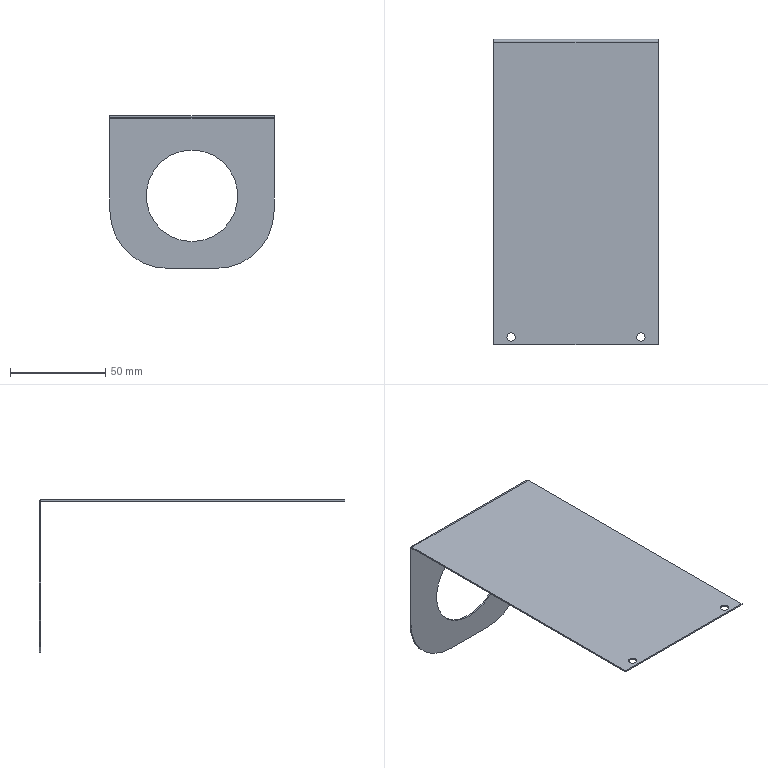Part | SolidWorks | features ICE 2, BreakCorner 1, FlatPattern 1, SMBaseFlange 1, SheetMetal 1 | 1 solid | 22 faces | box 86 x 160 x 80 mm | volume 13487 mm3 | plane 12 | cylinder 10 | commonest cylinder face diameters 4.4 x4 48 x2 60 x2 1.473 x1 2.946 x1
STEP:
#1=CARTESIAN_POINT('',(6.8,4.,-0.7366));
#2=VERTEX_POINT('',#1);
#3=CARTESIAN_POINT('',(11.2,4.,-0.7366));
#4=VERTEX_POINT('',#3);
#5=CARTESIAN_POINT('',(9.,4.,-0.7366));
#6=DIRECTION('',(0.,0.,1.));
#7=DIRECTION('',(1.,0.,0.));
#8=AXIS2_PLACEMENT_3D('',#5,#6,#7);
#9=CIRCLE('',#8,2.2);
#10=EDGE_CURVE('',#2,#4,#9,.T.);
#11=ORIENTED_EDGE('',*,*,#10,.F.);
#12=CARTESIAN_POINT('',(6.8,4.,0.));
#13=VERTEX_POINT('',#12);
#14=CARTESIAN_POINT('',(6.8,4.,-80.));
#15=DIRECTION('',(0.,0.,1.));
#16=VECTOR('',#15,1000.);
#17=LINE('',#14,#16);
#18=EDGE_CURVE('',#2,#13,#17,.T.);
#19=ORIENTED_EDGE('',*,*,#18,.T.);
#20=CARTESIAN_POINT('',(11.2,4.,0.));
#21=VERTEX_POINT('',#20);
#22=CARTESIAN_POINT('',(9.,4.,0.));
#23=DIRECTION('',(0.,0.,1.));
#24=DIRECTION('',(1.,0.,0.));
#25=AXIS2_PLACEMENT_3D('',#22,#23,#24);
#26=CIRCLE('',#25,2.2);
#27=EDGE_CURVE('',#13,#21,#26,.T.);
#28=ORIENTED_EDGE('',*,*,#27,.T.);
#29=CARTESIAN_POINT('',(11.2,4.,-80.));
#30=DIRECTION('',(0.,0.,1.));
#31=VECTOR('',#30,1000.);
#32=LINE('',#29,#31);
#33=EDGE_CURVE('',#4,#21,#32,.T.);
#34=ORIENTED_EDGE('',*,*,#33,.F.);
#35=EDGE_LOOP('',(#11,#19,#28,#34));
#36=FACE_OUTER_BOUND('',#35,.T.);
#37=CARTESIAN_POINT('',(9.,4.,-80.));
#38=DIRECTION('',(0.,0.,1.));
#39=DIRECTION('',(1.,0.,0.));
#40=AXIS2_PLACEMENT_3D('',#37,#38,#39);
#41=CYLINDRICAL_SURFACE('',#40,2.2);
#42=ADVANCED_FACE('',(#36),#41,.F.);
#43=CARTESIAN_POINT('',(74.8,4.,-0.7366));
#44=VERTEX_POINT('',#43);
#45=CARTESIAN_POINT('',(79.2,4.,-0.7366));
#46=VERTEX_POINT('',#45);
#47=CARTESIAN_POINT('',(77.,4.,-0.7366));
#48=DIRECTION('',(0.,0.,1.));
#49=DIRECTION('',(1.,0.,0.));
#50=AXIS2_PLACEMENT_3D('',#47,#48,#49);
#51=CIRCLE('',#50,2.2);
#52=EDGE_CURVE('',#44,#46,#51,.T.);
#53=ORIENTED_EDGE('',*,*,#52,.F.);
#54=CARTESIAN_POINT('',(74.8,4.,0.));
#55=VERTEX_POINT('',#54);
#56=CARTESIAN_POINT('',(74.8,4.,-80.));
#57=DIRECTION('',(0.,0.,1.));
#58=VECTOR('',#57,1000.);
#59=LINE('',#56,#58);
#60=EDGE_CURVE('',#44,#55,#59,.T.);
#61=ORIENTED_EDGE('',*,*,#60,.T.);
#62=CARTESIAN_POINT('',(79.2,4.,0.));
#63=VERTEX_POINT('',#62);
#64=CARTESIAN_POINT('',(77.,4.,0.));
#65=DIRECTION('',(0.,0.,1.));
#66=DIRECTION('',(1.,0.,0.));
#67=AXIS2_PLACEMENT_3D('',#64,#65,#66);
#68=CIRCLE('',#67,2.2);
#69=EDGE_CURVE('',#55,#63,#68,.T.);
#70=ORIENTED_EDGE('',*,*,#69,.T.);
#71=CARTESIAN_POINT('',(79.2,4.,-80.));
#72=DIRECTION('',(0.,0.,1.));
#73=VECTOR('',#72,1000.);
#74=LINE('',#71,#73);
#75=EDGE_CURVE('',#46,#63,#74,.T.);
#76=ORIENTED_EDGE('',*,*,#75,.F.);
#77=EDGE_LOOP('',(#53,#61,#70,#76));
#78=FACE_OUTER_BOUND('',#77,.T.);
#79=CARTESIAN_POINT('',(77.,4.,-80.));
#80=DIRECTION('',(0.,0.,1.));
#81=DIRECTION('',(1.,0.,0.));
#82=AXIS2_PLACEMENT_3D('',#79,#80,#81);
#83=CYLINDRICAL_SURFACE('',#82,2.2);
#84=ADVANCED_FACE('',(#78),#83,.F.);
#85=CARTESIAN_POINT('',(43.,159.263,-66.));
#86=VERTEX_POINT('',#85);
#87=CARTESIAN_POINT('',(43.,159.263,-18.));
#88=VERTEX_POINT('',#87);
#89=CARTESIAN_POINT('',(43.,159.263,-42.));
#90=DIRECTION('',(0.,1.,0.));
#91=DIRECTION('',(0.,0.,1.));
#92=AXIS2_PLACEMENT_3D('',#89,#90,#91);
#93=CIRCLE('',#92,24.);
#94=EDGE_CURVE('',#86,#88,#93,.T.);
#95=ORIENTED_EDGE('',*,*,#94,.F.);
#96=CARTESIAN_POINT('',(43.,160.,-66.));
#97=VERTEX_POINT('',#96);
#98=CARTESIAN_POINT('',(43.,150.,-66.));
#99=DIRECTION('',(0.,1.,0.));
#100=VECTOR('',#99,1000.);
#101=LINE('',#98,#100);
#102=EDGE_CURVE('',#86,#97,#101,.T.);
#103=ORIENTED_EDGE('',*,*,#102,.T.);
#104=CARTESIAN_POINT('',(43.,160.,-18.));
#105=VERTEX_POINT('',#104);
#106=CARTESIAN_POINT('',(43.,160.,-42.));
#107=DIRECTION('',(0.,1.,0.));
#108=DIRECTION('',(0.,0.,1.));
#109=AXIS2_PLACEMENT_3D('',#106,#107,#108);
#110=CIRCLE('',#109,24.);
#111=EDGE_CURVE('',#97,#105,#110,.T.);
#112=ORIENTED_EDGE('',*,*,#111,.T.);
#113=CARTESIAN_POINT('',(43.,150.,-18.));
#114=DIRECTION('',(0.,1.,0.));
#115=VECTOR('',#114,1000.);
#116=LINE('',#113,#115);
#117=EDGE_CURVE('',#88,#105,#116,.T.);
#118=ORIENTED_EDGE('',*,*,#117,.F.);
#119=EDGE_LOOP('',(#95,#103,#112,#118));
#120=FACE_OUTER_BOUND('',#119,.T.);
#121=CARTESIAN_POINT('',(43.,150.,-42.));
#122=DIRECTION('',(0.,1.,0.));
#123=DIRECTION('',(0.,0.,1.));
#124=AXIS2_PLACEMENT_3D('',#121,#122,#123);
#125=CYLINDRICAL_SURFACE('',#124,24.);
#126=ADVANCED_FACE('',(#120),#125,.F.);
#127=CARTESIAN_POINT('',(86.,160.,-1.473));
#128=VERTEX_POINT('',#127);
#129=CARTESIAN_POINT('',(86.,159.263,-1.473));
#130=VERTEX_POINT('',#129);
#131=CARTESIAN_POINT('',(86.,160.,-1.473));
#132=DIRECTION('',(0.,-1.,0.));
#133=VECTOR('',#132,1000.);
#134=LINE('',#131,#133);
#135=EDGE_CURVE('',#128,#130,#134,.T.);
#136=ORIENTED_EDGE('',*,*,#135,.F.);
#137=CARTESIAN_POINT('',(86.,158.527,0.));
#138=VERTEX_POINT('',#137);
#139=CARTESIAN_POINT('',(86.,158.527,-1.473));
#140=DIRECTION('',(-1.,0.,0.));
#141=DIRECTION('',(0.,0.,-1.));
#142=AXIS2_PLACEMENT_3D('',#139,#140,#141);
#143=CIRCLE('',#142,1.473);
#144=EDGE_CURVE('',#138,#128,#143,.T.);
#145=ORIENTED_EDGE('',*,*,#144,.F.);
#146=CARTESIAN_POINT('',(86.,158.527,-0.7366));
#147=VERTEX_POINT('',#146);
#148=CARTESIAN_POINT('',(86.,158.527,-0.7366));
#149=DIRECTION('',(0.,0.,1.));
#150=VECTOR('',#149,1000.);
#151=LINE('',#148,#150);
#152=EDGE_CURVE('',#147,#138,#151,.T.);
#153=ORIENTED_EDGE('',*,*,#152,.F.);
#154=CARTESIAN_POINT('',(86.,158.527,-1.473));
#155=DIRECTION('',(-1.,0.,0.));
#156=DIRECTION('',(0.,0.,-1.));
#157=AXIS2_PLACEMENT_3D('',#154,#155,#156);
#158=CIRCLE('',#157,0.7366);
#159=EDGE_CURVE('',#147,#130,#158,.T.);
#160=ORIENTED_EDGE('',*,*,#159,.T.);
#161=EDGE_LOOP('',(#136,#145,#153,#160));
#162=FACE_OUTER_BOUND('',#161,.T.);
#163=CARTESIAN_POINT('',(86.,160.,-1.473));
#164=DIRECTION('',(1.,0.,0.));
#165=DIRECTION('',(0.,0.,-1.));
#166=AXIS2_PLACEMENT_3D('',#163,#164,#165);
#167=PLANE('',#166);
#168=ADVANCED_FACE('',(#162),#167,.T.);
#169=CARTESIAN_POINT('',(86.,159.263,-50.));
#170=VERTEX_POINT('',#169);
#171=CARTESIAN_POINT('',(86.,159.263,0.));
#172=DIRECTION('',(0.,0.,-1.));
#173=VECTOR('',#172,1000.);
#174=LINE('',#171,#173);
#175=EDGE_CURVE('',#130,#170,#174,.T.);
#176=ORIENTED_EDGE('',*,*,#175,.T.);
#177=CARTESIAN_POINT('',(86.,160.,-50.));
#178=VERTEX_POINT('',#177);
#179=CARTESIAN_POINT('',(86.,158.527,-50.));
#180=DIRECTION('',(0.,1.,0.));
#181=VECTOR('',#180,1000.);
#182=LINE('',#179,#181);
#183=EDGE_CURVE('',#170,#178,#182,.T.);
#184=ORIENTED_EDGE('',*,*,#183,.T.);
#185=CARTESIAN_POINT('',(86.,160.,0.));
#186=DIRECTION('',(0.,0.,-1.));
#187=VECTOR('',#186,1000.);
#188=LINE('',#185,#187);
#189=EDGE_CURVE('',#128,#178,#188,.T.);
#190=ORIENTED_EDGE('',*,*,#189,.F.);
#191=ORIENTED_EDGE('',*,*,#135,.T.);
#192=EDGE_LOOP('',(#176,#184,#190,#191));
#193=FACE_OUTER_BOUND('',#192,.T.);
#194=CARTESIAN_POINT('',(86.,158.527,-0.7366));
#195=DIRECTION('',(1.,0.,0.));
#196=DIRECTION('',(0.,0.,-1.));
#197=AXIS2_PLACEMENT_3D('',#194,#195,#196);
#198=PLANE('',#197);
#199=ADVANCED_FACE('',(#193),#198,.T.);
#200=CARTESIAN_POINT('',(0.,158.527,0.));
#201=VERTEX_POINT('',#200);
#202=CARTESIAN_POINT('',(0.,158.527,-0.7366));
#203=VERTEX_POINT('',#202);
#204=CARTESIAN_POINT('',(0.,158.527,0.));
#205=DIRECTION('',(0.,0.,-1.));
#206=VECTOR('',#205,1000.);
#207=LINE('',#204,#206);
#208=EDGE_CURVE('',#201,#203,#207,.T.);
#209=ORIENTED_EDGE('',*,*,#208,.F.);
#210=CARTESIAN_POINT('',(0.,160.,-1.473));
#211=VERTEX_POINT('',#210);
#212=CARTESIAN_POINT('',(0.,158.527,-1.473));
#213=DIRECTION('',(-1.,0.,0.));
#214=DIRECTION('',(0.,0.,-1.));
#215=AXIS2_PLACEMENT_3D('',#212,#213,#214);
#216=CIRCLE('',#215,1.473);
#217=EDGE_CURVE('',#201,#211,#216,.T.);
#218=ORIENTED_EDGE('',*,*,#217,.T.);
#219=CARTESIAN_POINT('',(0.,159.263,-1.473));
#220=VERTEX_POINT('',#219);
#221=CARTESIAN_POINT('',(0.,159.263,-1.473));
#222=DIRECTION('',(0.,1.,0.));
#223=VECTOR('',#222,1000.);
#224=LINE('',#221,#223);
#225=EDGE_CURVE('',#220,#211,#224,.T.);
#226=ORIENTED_EDGE('',*,*,#225,.F.);
#227=CARTESIAN_POINT('',(0.,158.527,-1.473));
#228=DIRECTION('',(-1.,0.,0.));
#229=DIRECTION('',(0.,0.,-1.));
#230=AXIS2_PLACEMENT_3D('',#227,#228,#229);
#231=CIRCLE('',#230,0.7366);
#232=EDGE_CURVE('',#203,#220,#231,.T.);
#233=ORIENTED_EDGE('',*,*,#232,.F.);
#234=EDGE_LOOP('',(#209,#218,#226,#233));
#235=FACE_OUTER_BOUND('',#234,.T.);
#236=CARTESIAN_POINT('',(0.,158.527,0.));
#237=DIRECTION('',(-1.,0.,0.));
#238=DIRECTION('',(0.,0.,1.));
#239=AXIS2_PLACEMENT_3D('',#236,#237,#238);
#240=PLANE('',#239);
#241=ADVANCED_FACE('',(#235),#240,.T.);
#242=CARTESIAN_POINT('',(0.,0.,0.));
#243=VERTEX_POINT('',#242);
#244=CARTESIAN_POINT('',(0.,0.,0.));
#245=DIRECTION('',(0.,1.,0.));
#246=VECTOR('',#245,1000.);
#247=LINE('',#244,#246);
#248=EDGE_CURVE('',#243,#201,#247,.T.);
#249=ORIENTED_EDGE('',*,*,#248,.T.);
#250=ORIENTED_EDGE('',*,*,#208,.T.);
#251=CARTESIAN_POINT('',(0.,0.,-0.7366));
#252=VERTEX_POINT('',#251);
#253=CARTESIAN_POINT('',(0.,0.,-0.7366));
#254=DIRECTION('',(0.,1.,0.));
#255=VECTOR('',#254,1000.);
#256=LINE('',#253,#255);
#257=EDGE_CURVE('',#252,#203,#256,.T.);
#258=ORIENTED_EDGE('',*,*,#257,.F.);
#259=CARTESIAN_POINT('',(0.,0.,-0.7366));
#260=DIRECTION('',(0.,0.,1.));
#261=VECTOR('',#260,1000.);
#262=LINE('',#259,#261);
#263=EDGE_CURVE('',#252,#243,#262,.T.);
#264=ORIENTED_EDGE('',*,*,#263,.T.);
#265=EDGE_LOOP('',(#249,#250,#258,#264));
#266=FACE_OUTER_BOUND('',#265,.T.);
#267=CARTESIAN_POINT('',(0.,159.263,-1.473));
#268=DIRECTION('',(-1.,0.,0.));
#269=DIRECTION('',(0.,0.,1.));
#270=AXIS2_PLACEMENT_3D('',#267,#268,#269);
#271=PLANE('',#270);
#272=ADVANCED_FACE('',(#266),#271,.T.);
#273=CARTESIAN_POINT('',(43.,159.263,-42.));
#274=DIRECTION('',(0.,1.,0.));
#275=DIRECTION('',(0.,0.,1.));
#276=AXIS2_PLACEMENT_3D('',#273,#274,#275);
#277=CIRCLE('',#276,24.);
#278=EDGE_CURVE('',#88,#86,#277,.T.);
#279=ORIENTED_EDGE('',*,*,#278,.T.);
#280=ORIENTED_EDGE('',*,*,#94,.T.);
#281=EDGE_LOOP('',(#279,#280));
#282=FACE_BOUND('',#281,.T.);
#283=CARTESIAN_POINT('',(56.,159.263,-80.));
#284=VERTEX_POINT('',#283);
#285=CARTESIAN_POINT('',(30.,159.263,-80.));
#286=VERTEX_POINT('',#285);
#287=CARTESIAN_POINT('',(86.,159.263,-80.));
#288=DIRECTION('',(-1.,0.,0.));
#289=VECTOR('',#288,1000.);
#290=LINE('',#287,#289);
#291=EDGE_CURVE('',#284,#286,#290,.T.);
#292=ORIENTED_EDGE('',*,*,#291,.F.);
#293=CARTESIAN_POINT('',(56.,159.263,-50.));
#294=DIRECTION('',(0.,-1.,0.));
#295=DIRECTION('',(0.,0.,1.));
#296=AXIS2_PLACEMENT_3D('',#293,#294,#295);
#297=CIRCLE('',#296,30.);
#298=EDGE_CURVE('',#284,#170,#297,.T.);
#299=ORIENTED_EDGE('',*,*,#298,.T.);
#300=ORIENTED_EDGE('',*,*,#175,.F.);
#301=CARTESIAN_POINT('',(86.,159.263,-1.473));
#302=DIRECTION('',(-1.,0.,0.));
#303=VECTOR('',#302,1000.);
#304=LINE('',#301,#303);
#305=EDGE_CURVE('',#130,#220,#304,.T.);
#306=ORIENTED_EDGE('',*,*,#305,.T.);
#307=CARTESIAN_POINT('',(0.,159.263,-50.));
#308=VERTEX_POINT('',#307);
#309=CARTESIAN_POINT('',(0.,159.263,0.));
#310=DIRECTION('',(0.,0.,-1.));
#311=VECTOR('',#310,1000.);
#312=LINE('',#309,#311);
#313=EDGE_CURVE('',#220,#308,#312,.T.);
#314=ORIENTED_EDGE('',*,*,#313,.T.);
#315=CARTESIAN_POINT('',(30.,159.263,-50.));
#316=DIRECTION('',(0.,-1.,0.));
#317=DIRECTION('',(0.,0.,1.));
#318=AXIS2_PLACEMENT_3D('',#315,#316,#317);
#319=CIRCLE('',#318,30.);
#320=EDGE_CURVE('',#308,#286,#319,.T.);
#321=ORIENTED_EDGE('',*,*,#320,.T.);
#322=EDGE_LOOP('',(#292,#299,#300,#306,#314,#321));
#323=FACE_OUTER_BOUND('',#322,.T.);
#324=CARTESIAN_POINT('',(86.,159.263,0.));
#325=DIRECTION('',(0.,1.,0.));
#326=DIRECTION('',(0.,0.,1.));
#327=AXIS2_PLACEMENT_3D('',#324,#325,#326);
#328=PLANE('',#327);
#329=ADVANCED_FACE('',(#282,#323),#328,.F.);
#330=CARTESIAN_POINT('',(56.,160.,-80.));
#331=VERTEX_POINT('',#330);
#332=CARTESIAN_POINT('',(30.,160.,-80.));
#333=VERTEX_POINT('',#332);
#334=CARTESIAN_POINT('',(86.,160.,-80.));
#335=DIRECTION('',(-1.,0.,0.));
#336=VECTOR('',#335,1000.);
#337=LINE('',#334,#336);
#338=EDGE_CURVE('',#331,#333,#337,.T.);
#339=ORIENTED_EDGE('',*,*,#338,.F.);
#340=CARTESIAN_POINT('',(56.,160.,-80.));
#341=DIRECTION('',(0.,-1.,0.));
#342=VECTOR('',#341,1000.);
#343=LINE('',#340,#342);
#344=EDGE_CURVE('',#331,#284,#343,.T.);
#345=ORIENTED_EDGE('',*,*,#344,.T.);
#346=ORIENTED_EDGE('',*,*,#291,.T.);
#347=CARTESIAN_POINT('',(30.,160.,-80.));
#348=DIRECTION('',(0.,1.,0.));
#349=VECTOR('',#348,1000.);
#350=LINE('',#347,#349);
#351=EDGE_CURVE('',#286,#333,#350,.T.);
#352=ORIENTED_EDGE('',*,*,#351,.T.);
#353=EDGE_LOOP('',(#339,#345,#346,#352));
#354=FACE_OUTER_BOUND('',#353,.T.);
#355=CARTESIAN_POINT('',(86.,160.,-80.));
#356=DIRECTION('',(0.,0.,-1.));
#357=DIRECTION('',(-1.,0.,0.));
#358=AXIS2_PLACEMENT_3D('',#355,#356,#357);
#359=PLANE('',#358);
#360=ADVANCED_FACE('',(#354),#359,.T.);
#361=CARTESIAN_POINT('',(43.,160.,-42.));
#362=DIRECTION('',(0.,1.,0.));
#363=DIRECTION('',(0.,0.,1.));
#364=AXIS2_PLACEMENT_3D('',#361,#362,#363);
#365=CIRCLE('',#364,24.);
#366=EDGE_CURVE('',#105,#97,#365,.T.);
#367=ORIENTED_EDGE('',*,*,#366,.F.);
#368=ORIENTED_EDGE('',*,*,#111,.F.);
#369=EDGE_LOOP('',(#367,#368));
#370=FACE_BOUND('',#369,.T.);
#371=ORIENTED_EDGE('',*,*,#189,.T.);
#372=CARTESIAN_POINT('',(56.,160.,-50.));
#373=DIRECTION('',(0.,1.,0.));
#374=DIRECTION('',(0.,0.,1.));
#375=AXIS2_PLACEMENT_3D('',#372,#373,#374);
#376=CIRCLE('',#375,30.);
#377=EDGE_CURVE('',#178,#331,#376,.T.);
#378=ORIENTED_EDGE('',*,*,#377,.T.);
#379=ORIENTED_EDGE('',*,*,#338,.T.);
#380=CARTESIAN_POINT('',(0.,160.,-50.));
#381=VERTEX_POINT('',#380);
#382=CARTESIAN_POINT('',(30.,160.,-50.));
#383=DIRECTION('',(0.,1.,0.));
#384=DIRECTION('',(0.,0.,1.));
#385=AXIS2_PLACEMENT_3D('',#382,#383,#384);
#386=CIRCLE('',#385,30.);
#387=EDGE_CURVE('',#333,#381,#386,.T.);
#388=ORIENTED_EDGE('',*,*,#387,.T.);
#389=CARTESIAN_POINT('',(0.,160.,0.));
#390=DIRECTION('',(0.,0.,-1.));
#391=VECTOR('',#390,1000.);
#392=LINE('',#389,#391);
#393=EDGE_CURVE('',#211,#381,#392,.T.);
#394=ORIENTED_EDGE('',*,*,#393,.F.);
#395=CARTESIAN_POINT('',(86.,160.,-1.473));
#396=DIRECTION('',(-1.,0.,0.));
#397=VECTOR('',#396,1000.);
#398=LINE('',#395,#397);
#399=EDGE_CURVE('',#128,#211,#398,.T.);
#400=ORIENTED_EDGE('',*,*,#399,.F.);
#401=EDGE_LOOP('',(#371,#378,#379,#388,#394,#400));
#402=FACE_OUTER_BOUND('',#401,.T.);
#403=CARTESIAN_POINT('',(86.,160.,0.));
#404=DIRECTION('',(0.,1.,0.));
#405=DIRECTION('',(0.,0.,1.));
#406=AXIS2_PLACEMENT_3D('',#403,#404,#405);
#407=PLANE('',#406);
#408=ADVANCED_FACE('',(#370,#402),#407,.T.);
#409=ORIENTED_EDGE('',*,*,#217,.F.);
#410=CARTESIAN_POINT('',(86.,158.527,0.));
#411=DIRECTION('',(-1.,0.,0.));
#412=VECTOR('',#411,1000.);
#413=LINE('',#410,#412);
#414=EDGE_CURVE('',#138,#201,#413,.T.);
#415=ORIENTED_EDGE('',*,*,#414,.F.);
#416=ORIENTED_EDGE('',*,*,#144,.T.);
#417=ORIENTED_EDGE('',*,*,#399,.T.);
#418=EDGE_LOOP('',(#409,#415,#416,#417));
#419=FACE_OUTER_BOUND('',#418,.T.);
#420=CARTESIAN_POINT('',(86.,158.527,-1.473));
#421=DIRECTION('',(-1.,0.,0.));
#422=DIRECTION('',(0.,0.,1.));
#423=AXIS2_PLACEMENT_3D('',#420,#421,#422);
#424=CYLINDRICAL_SURFACE('',#423,1.473);
#425=ADVANCED_FACE('',(#419),#424,.T.);
#426=CARTESIAN_POINT('',(9.,4.,0.));
#427=DIRECTION('',(0.,0.,1.));
#428=DIRECTION('',(1.,0.,0.));
#429=AXIS2_PLACEMENT_3D('',#426,#427,#428);
#430=CIRCLE('',#429,2.2);
#431=EDGE_CURVE('',#21,#13,#430,.T.);
#432=ORIENTED_EDGE('',*,*,#431,.F.);
#433=ORIENTED_EDGE('',*,*,#27,.F.);
#434=EDGE_LOOP('',(#432,#433));
#435=FACE_BOUND('',#434,.T.);
#436=CARTESIAN_POINT('',(77.,4.,0.));
#437=DIRECTION('',(0.,0.,1.));
#438=DIRECTION('',(1.,0.,0.));
#439=AXIS2_PLACEMENT_3D('',#436,#437,#438);
#440=CIRCLE('',#439,2.2);
#441=EDGE_CURVE('',#63,#55,#440,.T.);
#442=ORIENTED_EDGE('',*,*,#441,.F.);
#443=ORIENTED_EDGE('',*,*,#69,.F.);
#444=EDGE_LOOP('',(#442,#443));
#445=FACE_BOUND('',#444,.T.);
#446=ORIENTED_EDGE('',*,*,#248,.F.);
#447=CARTESIAN_POINT('',(86.,0.,0.));
#448=VERTEX_POINT('',#447);
#449=CARTESIAN_POINT('',(86.,0.,0.));
#450=DIRECTION('',(-1.,0.,0.));
#451=VECTOR('',#450,1000.);
#452=LINE('',#449,#451);
#453=EDGE_CURVE('',#448,#243,#452,.T.);
#454=ORIENTED_EDGE('',*,*,#453,.F.);
#455=CARTESIAN_POINT('',(86.,0.,0.));
#456=DIRECTION('',(0.,1.,0.));
#457=VECTOR('',#456,1000.);
#458=LINE('',#455,#457);
#459=EDGE_CURVE('',#448,#138,#458,.T.);
#460=ORIENTED_EDGE('',*,*,#459,.T.);
#461=ORIENTED_EDGE('',*,*,#414,.T.);
#462=EDGE_LOOP('',(#446,#454,#460,#461));
#463=FACE_OUTER_BOUND('',#462,.T.);
#464=CARTESIAN_POINT('',(86.,0.,0.));
#465=DIRECTION('',(0.,0.,1.));
#466=DIRECTION('',(1.,0.,0.));
#467=AXIS2_PLACEMENT_3D('',#464,#465,#466);
#468=PLANE('',#467);
#469=ADVANCED_FACE('',(#435,#445,#463),#468,.T.);
#470=ORIENTED_EDGE('',*,*,#263,.F.);
#471=CARTESIAN_POINT('',(86.,0.,-0.7366));
#472=VERTEX_POINT('',#471);
#473=CARTESIAN_POINT('',(86.,0.,-0.7366));
#474=DIRECTION('',(-1.,0.,0.));
#475=VECTOR('',#474,1000.);
#476=LINE('',#473,#475);
#477=EDGE_CURVE('',#472,#252,#476,.T.);
#478=ORIENTED_EDGE('',*,*,#477,.F.);
#479=CARTESIAN_POINT('',(86.,0.,-0.7366));
#480=DIRECTION('',(0.,0.,1.));
#481=VECTOR('',#480,1000.);
#482=LINE('',#479,#481);
#483=EDGE_CURVE('',#472,#448,#482,.T.);
#484=ORIENTED_EDGE('',*,*,#483,.T.);
#485=ORIENTED_EDGE('',*,*,#453,.T.);
#486=EDGE_LOOP('',(#470,#478,#484,#485));
#487=FACE_OUTER_BOUND('',#486,.T.);
#488=CARTESIAN_POINT('',(86.,0.,-0.7366));
#489=DIRECTION('',(0.,-1.,0.));
#490=DIRECTION('',(0.,0.,-1.));
#491=AXIS2_PLACEMENT_3D('',#488,#489,#490);
#492=PLANE('',#491);
#493=ADVANCED_FACE('',(#487),#492,.T.);
#494=CARTESIAN_POINT('',(9.,4.,-0.7366));
#495=DIRECTION('',(0.,0.,1.));
#496=DIRECTION('',(1.,0.,0.));
#497=AXIS2_PLACEMENT_3D('',#494,#495,#496);
#498=CIRCLE('',#497,2.2);
#499=EDGE_CURVE('',#4,#2,#498,.T.);
#500=ORIENTED_EDGE('',*,*,#499,.T.);
#501=ORIENTED_EDGE('',*,*,#10,.T.);
#502=EDGE_LOOP('',(#500,#501));
#503=FACE_BOUND('',#502,.T.);
#504=CARTESIAN_POINT('',(77.,4.,-0.7366));
#505=DIRECTION('',(0.,0.,1.));
#506=DIRECTION('',(1.,0.,0.));
#507=AXIS2_PLACEMENT_3D('',#504,#505,#506);
#508=CIRCLE('',#507,2.2);
#509=EDGE_CURVE('',#46,#44,#508,.T.);
#510=ORIENTED_EDGE('',*,*,#509,.T.);
#511=ORIENTED_EDGE('',*,*,#52,.T.);
#512=EDGE_LOOP('',(#510,#511));
#513=FACE_BOUND('',#512,.T.);
#514=ORIENTED_EDGE('',*,*,#257,.T.);
#515=CARTESIAN_POINT('',(86.,158.527,-0.7366));
#516=DIRECTION('',(-1.,0.,0.));
#517=VECTOR('',#516,1000.);
#518=LINE('',#515,#517);
#519=EDGE_CURVE('',#147,#203,#518,.T.);
#520=ORIENTED_EDGE('',*,*,#519,.F.);
#521=CARTESIAN_POINT('',(86.,0.,-0.7366));
#522=DIRECTION('',(0.,1.,0.));
#523=VECTOR('',#522,1000.);
#524=LINE('',#521,#523);
#525=EDGE_CURVE('',#472,#147,#524,.T.);
#526=ORIENTED_EDGE('',*,*,#525,.F.);
#527=ORIENTED_EDGE('',*,*,#477,.T.);
#528=EDGE_LOOP('',(#514,#520,#526,#527));
#529=FACE_OUTER_BOUND('',#528,.T.);
#530=CARTESIAN_POINT('',(86.,0.,-0.7366));
#531=DIRECTION('',(0.,0.,1.));
#532=DIRECTION('',(1.,0.,0.));
#533=AXIS2_PLACEMENT_3D('',#530,#531,#532);
#534=PLANE('',#533);
#535=ADVANCED_FACE('',(#503,#513,#529),#534,.F.);
#536=ORIENTED_EDGE('',*,*,#232,.T.);
#537=ORIENTED_EDGE('',*,*,#305,.F.);
#538=ORIENTED_EDGE('',*,*,#159,.F.);
#539=ORIENTED_EDGE('',*,*,#519,.T.);
#540=EDGE_LOOP('',(#536,#537,#538,#539));
#541=FACE_OUTER_BOUND('',#540,.T.);
#542=CARTESIAN_POINT('',(86.,158.527,-1.473));
#543=DIRECTION('',(-1.,0.,0.));
#544=DIRECTION('',(0.,0.,1.));
#545=AXIS2_PLACEMENT_3D('',#542,#543,#544);
#546=CYLINDRICAL_SURFACE('',#545,0.7366);
#547=ADVANCED_FACE('',(#541),#546,.F.);
#548=ORIENTED_EDGE('',*,*,#525,.T.);
#549=ORIENTED_EDGE('',*,*,#152,.T.);
#550=ORIENTED_EDGE('',*,*,#459,.F.);
#551=ORIENTED_EDGE('',*,*,#483,.F.);
#552=EDGE_LOOP('',(#548,#549,#550,#551));
#553=FACE_OUTER_BOUND('',#552,.T.);
#554=CARTESIAN_POINT('',(86.,158.527,-1.473));
#555=DIRECTION('',(1.,0.,0.));
#556=DIRECTION('',(0.,0.,-1.));
#557=AXIS2_PLACEMENT_3D('',#554,#555,#556);
#558=PLANE('',#557);
#559=ADVANCED_FACE('',(#553),#558,.T.);
#560=ORIENTED_EDGE('',*,*,#393,.T.);
#561=CARTESIAN_POINT('',(0.,159.263,-50.));
#562=DIRECTION('',(0.,-1.,0.));
#563=VECTOR('',#562,1000.);
#564=LINE('',#561,#563);
#565=EDGE_CURVE('',#381,#308,#564,.T.);
#566=ORIENTED_EDGE('',*,*,#565,.T.);
#567=ORIENTED_EDGE('',*,*,#313,.F.);
#568=ORIENTED_EDGE('',*,*,#225,.T.);
#569=EDGE_LOOP('',(#560,#566,#567,#568));
#570=FACE_OUTER_BOUND('',#569,.T.);
#571=CARTESIAN_POINT('',(0.,158.527,-1.473));
#572=DIRECTION('',(1.,0.,0.));
#573=DIRECTION('',(0.,0.,-1.));
#574=AXIS2_PLACEMENT_3D('',#571,#572,#573);
#575=PLANE('',#574);
#576=ADVANCED_FACE('',(#570),#575,.F.);
#577=ORIENTED_EDGE('',*,*,#102,.F.);
#578=ORIENTED_EDGE('',*,*,#278,.F.);
#579=ORIENTED_EDGE('',*,*,#117,.T.);
#580=ORIENTED_EDGE('',*,*,#366,.T.);
#581=EDGE_LOOP('',(#577,#578,#579,#580));
#582=FACE_OUTER_BOUND('',#581,.T.);
#583=CARTESIAN_POINT('',(43.,150.,-42.));
#584=DIRECTION('',(0.,1.,0.));
#585=DIRECTION('',(0.,0.,1.));
#586=AXIS2_PLACEMENT_3D('',#583,#584,#585);
#587=CYLINDRICAL_SURFACE('',#586,24.);
#588=ADVANCED_FACE('',(#582),#587,.F.);
#589=ORIENTED_EDGE('',*,*,#377,.F.);
#590=ORIENTED_EDGE('',*,*,#183,.F.);
#591=ORIENTED_EDGE('',*,*,#298,.F.);
#592=ORIENTED_EDGE('',*,*,#344,.F.);
#593=EDGE_LOOP('',(#589,#590,#591,#592));
#594=FACE_OUTER_BOUND('',#593,.T.);
#595=CARTESIAN_POINT('',(56.,160.,-50.));
#596=DIRECTION('',(0.,-1.,0.));
#597=DIRECTION('',(0.,0.,-1.));
#598=AXIS2_PLACEMENT_3D('',#595,#596,#597);
#599=CYLINDRICAL_SURFACE('',#598,30.);
#600=ADVANCED_FACE('',(#594),#599,.T.);
#601=ORIENTED_EDGE('',*,*,#387,.F.);
#602=ORIENTED_EDGE('',*,*,#351,.F.);
#603=ORIENTED_EDGE('',*,*,#320,.F.);
#604=ORIENTED_EDGE('',*,*,#565,.F.);
#605=EDGE_LOOP('',(#601,#602,#603,#604));
#606=FACE_OUTER_BOUND('',#605,.T.);
#607=CARTESIAN_POINT('',(30.,158.527,-50.));
#608=DIRECTION('',(0.,1.,0.));
#609=DIRECTION('',(0.,0.,1.));
#610=AXIS2_PLACEMENT_3D('',#607,#608,#609);
#611=CYLINDRICAL_SURFACE('',#610,30.);
#612=ADVANCED_FACE('',(#606),#611,.T.);
#613=ORIENTED_EDGE('',*,*,#60,.F.);
#614=ORIENTED_EDGE('',*,*,#509,.F.);
#615=ORIENTED_EDGE('',*,*,#75,.T.);
#616=ORIENTED_EDGE('',*,*,#441,.T.);
#617=EDGE_LOOP('',(#613,#614,#615,#616));
#618=FACE_OUTER_BOUND('',#617,.T.);
#619=CARTESIAN_POINT('',(77.,4.,-80.));
#620=DIRECTION('',(0.,0.,1.));
#621=DIRECTION('',(1.,0.,0.));
#622=AXIS2_PLACEMENT_3D('',#619,#620,#621);
#623=CYLINDRICAL_SURFACE('',#622,2.2);
#624=ADVANCED_FACE('',(#618),#623,.F.);
#625=ORIENTED_EDGE('',*,*,#18,.F.);
#626=ORIENTED_EDGE('',*,*,#499,.F.);
#627=ORIENTED_EDGE('',*,*,#33,.T.);
#628=ORIENTED_EDGE('',*,*,#431,.T.);
#629=EDGE_LOOP('',(#625,#626,#627,#628));
#630=FACE_OUTER_BOUND('',#629,.T.);
#631=CARTESIAN_POINT('',(9.,4.,-80.));
#632=DIRECTION('',(0.,0.,1.));
#633=DIRECTION('',(1.,0.,0.));
#634=AXIS2_PLACEMENT_3D('',#631,#632,#633);
#635=CYLINDRICAL_SURFACE('',#634,2.2);
#636=ADVANCED_FACE('',(#630),#635,.F.);
#637=CLOSED_SHELL('',(#42,#84,#126,#168,#199,#241,#272,#329,#360,#408,#425,#469,#493,#535,#547,#559,#576,#588,#600,#612,#624,#636));
#638=MANIFOLD_SOLID_BREP('',#637);
#639=CARTESIAN_POINT('',(0.,0.,0.));
#640=DIRECTION('',(0.,0.,1.));
#641=DIRECTION('',(1.,0.,0.));
#642=AXIS2_PLACEMENT_3D('',#639,#640,#641);
#643=(LENGTH_UNIT()NAMED_UNIT(*)SI_UNIT(.MILLI.,.METRE.));
#644=UNCERTAINTY_MEASURE_WITH_UNIT(LENGTH_MEASURE(0.00001),#643,'','');
#645=(NAMED_UNIT(*)PLANE_ANGLE_UNIT()SI_UNIT($,.RADIAN.));
#646=(NAMED_UNIT(*)SI_UNIT($,.STERADIAN.)SOLID_ANGLE_UNIT());
#647=(GEOMETRIC_REPRESENTATION_CONTEXT(3)GLOBAL_UNCERTAINTY_ASSIGNED_CONTEXT((#644))GLOBAL_UNIT_ASSIGNED_CONTEXT((#643,#645,#646))REPRESENTATION_CONTEXT('',''));
#648=ADVANCED_BREP_SHAPE_REPRESENTATION('',(#638,#642),#647);